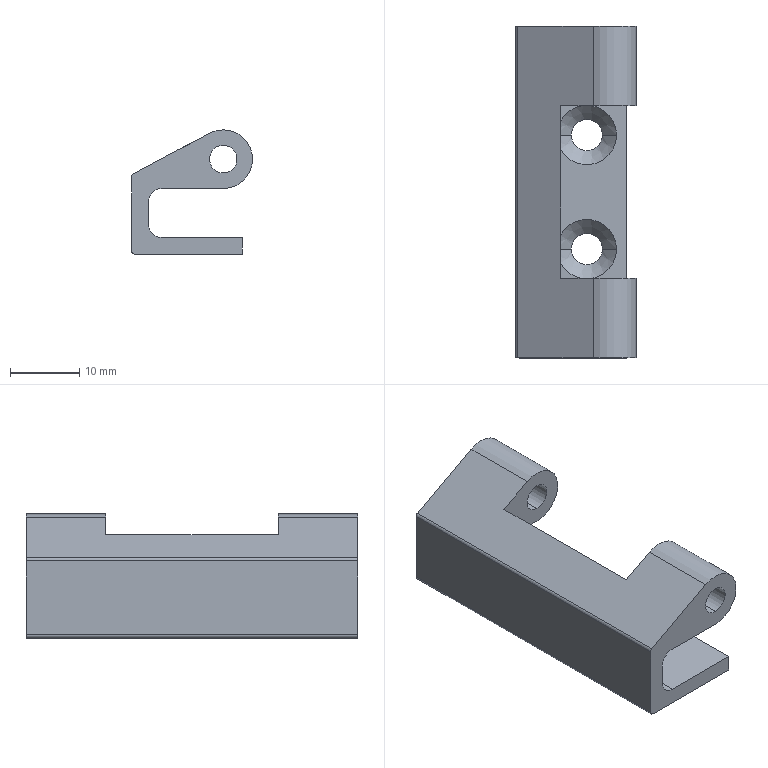Part | STEP file | Hinge CL237Z3H001-01 | 1 solid | 30 faces | box 17.5 x 48 x 18 mm | volume 5234 mm3 | cylinder 14 | plane 12 | cone 4 | commonest cylinder face diameters 4 x6 4.5 x4 1 x2 8.5 x2